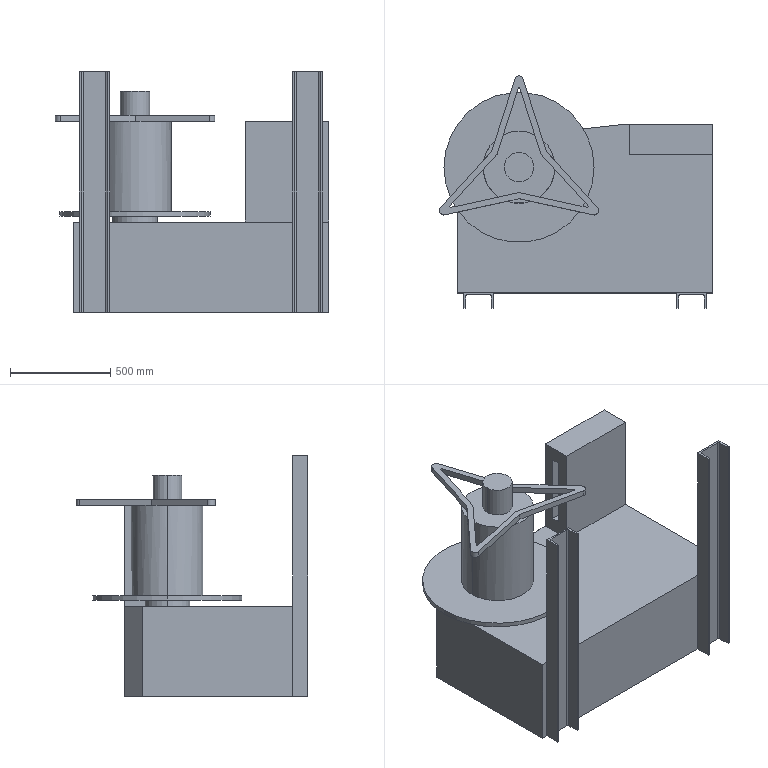Part | Creo | features CURVE 11, PROTRUSION 10, CUT 4, DATUM PLANE 3, ROUND 2, COORDINATE SYSTEM 1, MIRROR 1, PATTERN 1 | 1 solid | 87 faces | volume 559581150 mm3 | plane 69 | cylinder 18 | commonest cylinder face diameters 15 x4 9 x3 45 x3 147 x2 225 x2 360 x2